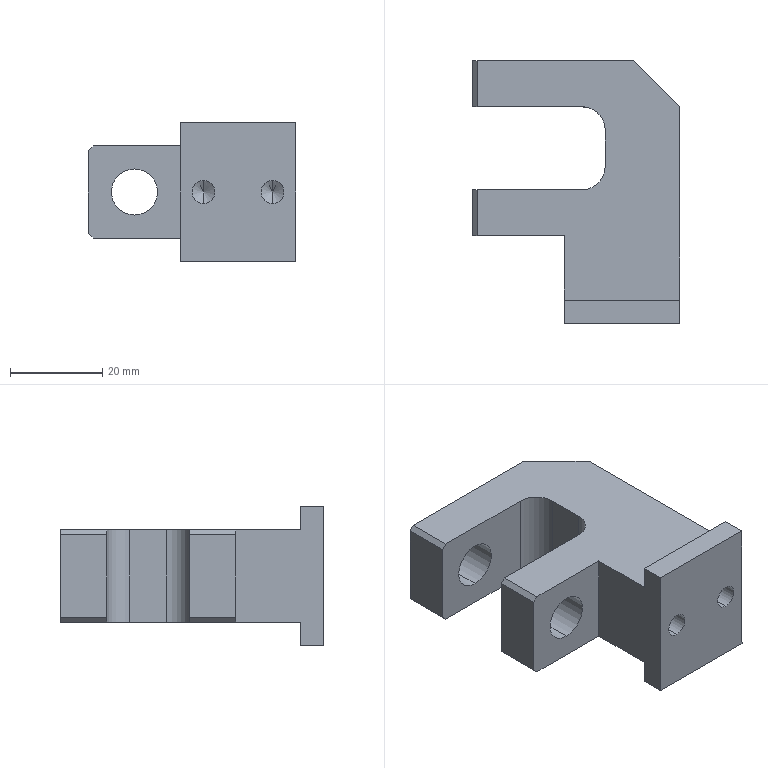Part | SolidWorks | features ICE 4, HoleWzd 3, Chamfer 2, Extrusion 1, Fillet 1 | 1 solid | 35 faces | box 45 x 57 x 30 mm | volume 31506 mm3 | plane 21 | cylinder 10 | cone 4 | commonest cylinder face diameters 10 x6 5 x4
STEP:
#1=CARTESIAN_POINT('',(-2.855,17.,2.5));
#2=VERTEX_POINT('',#1);
#3=CARTESIAN_POINT('',(-2.855,17.,-2.5));
#4=VERTEX_POINT('',#3);
#5=CARTESIAN_POINT('',(-2.855,17.,0.));
#6=DIRECTION('',(0.,-1.,0.));
#7=DIRECTION('',(0.,0.,-1.));
#8=AXIS2_PLACEMENT_3D('',#5,#6,#7);
#9=CIRCLE('',#8,2.5);
#10=EDGE_CURVE('',#2,#4,#9,.T.);
#11=ORIENTED_EDGE('',*,*,#10,.F.);
#12=CARTESIAN_POINT('',(-2.855,0.,2.5));
#13=VERTEX_POINT('',#12);
#14=CARTESIAN_POINT('',(-2.855,0.,2.5));
#15=DIRECTION('',(0.,-1.,0.));
#16=VECTOR('',#15,1000.);
#17=LINE('',#14,#16);
#18=EDGE_CURVE('',#2,#13,#17,.T.);
#19=ORIENTED_EDGE('',*,*,#18,.T.);
#20=CARTESIAN_POINT('',(-2.855,0.,-2.5));
#21=VERTEX_POINT('',#20);
#22=CARTESIAN_POINT('',(-2.855,0.,0.));
#23=DIRECTION('',(0.,-1.,0.));
#24=DIRECTION('',(0.,0.,-1.));
#25=AXIS2_PLACEMENT_3D('',#22,#23,#24);
#26=CIRCLE('',#25,2.5);
#27=EDGE_CURVE('',#13,#21,#26,.T.);
#28=ORIENTED_EDGE('',*,*,#27,.T.);
#29=CARTESIAN_POINT('',(-2.855,0.,-2.5));
#30=DIRECTION('',(0.,-1.,0.));
#31=VECTOR('',#30,1000.);
#32=LINE('',#29,#31);
#33=EDGE_CURVE('',#4,#21,#32,.T.);
#34=ORIENTED_EDGE('',*,*,#33,.F.);
#35=EDGE_LOOP('',(#11,#19,#28,#34));
#36=FACE_OUTER_BOUND('',#35,.T.);
#37=CARTESIAN_POINT('',(-2.855,0.,0.));
#38=DIRECTION('',(0.,-1.,0.));
#39=DIRECTION('',(0.,0.,-1.));
#40=AXIS2_PLACEMENT_3D('',#37,#38,#39);
#41=CYLINDRICAL_SURFACE('',#40,2.5);
#42=ADVANCED_FACE('',(#36),#41,.F.);
#43=CARTESIAN_POINT('',(-2.855,18.502,0.));
#44=VERTEX_POINT('',#43);
#45=CARTESIAN_POINT('',(-2.855,17.,-2.5));
#46=DIRECTION('',(0.,-0.515,-0.8572));
#47=VECTOR('',#46,1000.);
#48=LINE('',#45,#47);
#49=EDGE_CURVE('',#44,#4,#48,.T.);
#50=ORIENTED_EDGE('',*,*,#49,.F.);
#51=CARTESIAN_POINT('',(-2.855,17.,2.5));
#52=DIRECTION('',(0.,-0.515,0.8572));
#53=VECTOR('',#52,1000.);
#54=LINE('',#51,#53);
#55=EDGE_CURVE('',#44,#2,#54,.T.);
#56=ORIENTED_EDGE('',*,*,#55,.T.);
#57=ORIENTED_EDGE('',*,*,#10,.T.);
#58=EDGE_LOOP('',(#50,#56,#57));
#59=FACE_OUTER_BOUND('',#58,.T.);
#60=CARTESIAN_POINT('',(-2.855,17.,0.));
#61=DIRECTION('',(0.,-1.,0.));
#62=DIRECTION('',(0.,0.,-1.));
#63=AXIS2_PLACEMENT_3D('',#60,#61,#62);
#64=CONICAL_SURFACE('',#63,2.5,1.03);
#65=ADVANCED_FACE('',(#59),#64,.F.);
#66=CARTESIAN_POINT('',(12.145,17.,2.5));
#67=VERTEX_POINT('',#66);
#68=CARTESIAN_POINT('',(12.145,17.,-2.5));
#69=VERTEX_POINT('',#68);
#70=CARTESIAN_POINT('',(12.145,17.,0.));
#71=DIRECTION('',(0.,-1.,0.));
#72=DIRECTION('',(0.,0.,-1.));
#73=AXIS2_PLACEMENT_3D('',#70,#71,#72);
#74=CIRCLE('',#73,2.5);
#75=EDGE_CURVE('',#67,#69,#74,.T.);
#76=ORIENTED_EDGE('',*,*,#75,.F.);
#77=CARTESIAN_POINT('',(12.145,0.,2.5));
#78=VERTEX_POINT('',#77);
#79=CARTESIAN_POINT('',(12.145,0.,2.5));
#80=DIRECTION('',(0.,-1.,0.));
#81=VECTOR('',#80,1000.);
#82=LINE('',#79,#81);
#83=EDGE_CURVE('',#67,#78,#82,.T.);
#84=ORIENTED_EDGE('',*,*,#83,.T.);
#85=CARTESIAN_POINT('',(12.145,0.,-2.5));
#86=VERTEX_POINT('',#85);
#87=CARTESIAN_POINT('',(12.145,0.,0.));
#88=DIRECTION('',(0.,-1.,0.));
#89=DIRECTION('',(0.,0.,-1.));
#90=AXIS2_PLACEMENT_3D('',#87,#88,#89);
#91=CIRCLE('',#90,2.5);
#92=EDGE_CURVE('',#78,#86,#91,.T.);
#93=ORIENTED_EDGE('',*,*,#92,.T.);
#94=CARTESIAN_POINT('',(12.145,0.,-2.5));
#95=DIRECTION('',(0.,-1.,0.));
#96=VECTOR('',#95,1000.);
#97=LINE('',#94,#96);
#98=EDGE_CURVE('',#69,#86,#97,.T.);
#99=ORIENTED_EDGE('',*,*,#98,.F.);
#100=EDGE_LOOP('',(#76,#84,#93,#99));
#101=FACE_OUTER_BOUND('',#100,.T.);
#102=CARTESIAN_POINT('',(12.145,0.,0.));
#103=DIRECTION('',(0.,-1.,0.));
#104=DIRECTION('',(0.,0.,-1.));
#105=AXIS2_PLACEMENT_3D('',#102,#103,#104);
#106=CYLINDRICAL_SURFACE('',#105,2.5);
#107=ADVANCED_FACE('',(#101),#106,.F.);
#108=CARTESIAN_POINT('',(12.145,18.502,0.));
#109=VERTEX_POINT('',#108);
#110=CARTESIAN_POINT('',(12.145,17.,-2.5));
#111=DIRECTION('',(0.,-0.515,-0.8572));
#112=VECTOR('',#111,1000.);
#113=LINE('',#110,#112);
#114=EDGE_CURVE('',#109,#69,#113,.T.);
#115=ORIENTED_EDGE('',*,*,#114,.F.);
#116=CARTESIAN_POINT('',(12.145,17.,2.5));
#117=DIRECTION('',(0.,-0.515,0.8572));
#118=VECTOR('',#117,1000.);
#119=LINE('',#116,#118);
#120=EDGE_CURVE('',#109,#67,#119,.T.);
#121=ORIENTED_EDGE('',*,*,#120,.T.);
#122=ORIENTED_EDGE('',*,*,#75,.T.);
#123=EDGE_LOOP('',(#115,#121,#122));
#124=FACE_OUTER_BOUND('',#123,.T.);
#125=CARTESIAN_POINT('',(12.145,17.,0.));
#126=DIRECTION('',(0.,-1.,0.));
#127=DIRECTION('',(0.,0.,-1.));
#128=AXIS2_PLACEMENT_3D('',#125,#126,#127);
#129=CONICAL_SURFACE('',#128,2.5,1.03);
#130=ADVANCED_FACE('',(#124),#129,.F.);
#131=CARTESIAN_POINT('',(-17.855,29.,5.));
#132=VERTEX_POINT('',#131);
#133=CARTESIAN_POINT('',(-17.855,29.,-5.));
#134=VERTEX_POINT('',#133);
#135=CARTESIAN_POINT('',(-17.855,29.,0.));
#136=DIRECTION('',(0.,-1.,0.));
#137=DIRECTION('',(0.,0.,-1.));
#138=AXIS2_PLACEMENT_3D('',#135,#136,#137);
#139=CIRCLE('',#138,5.);
#140=EDGE_CURVE('',#132,#134,#139,.T.);
#141=ORIENTED_EDGE('',*,*,#140,.F.);
#142=CARTESIAN_POINT('',(-17.855,19.,5.));
#143=VERTEX_POINT('',#142);
#144=CARTESIAN_POINT('',(-17.855,19.,5.));
#145=DIRECTION('',(0.,-1.,0.));
#146=VECTOR('',#145,1000.);
#147=LINE('',#144,#146);
#148=EDGE_CURVE('',#132,#143,#147,.T.);
#149=ORIENTED_EDGE('',*,*,#148,.T.);
#150=CARTESIAN_POINT('',(-17.855,19.,-5.));
#151=VERTEX_POINT('',#150);
#152=CARTESIAN_POINT('',(-17.855,19.,0.));
#153=DIRECTION('',(0.,-1.,0.));
#154=DIRECTION('',(0.,0.,-1.));
#155=AXIS2_PLACEMENT_3D('',#152,#153,#154);
#156=CIRCLE('',#155,5.);
#157=EDGE_CURVE('',#143,#151,#156,.T.);
#158=ORIENTED_EDGE('',*,*,#157,.T.);
#159=CARTESIAN_POINT('',(-17.855,19.,-5.));
#160=DIRECTION('',(0.,-1.,0.));
#161=VECTOR('',#160,1000.);
#162=LINE('',#159,#161);
#163=EDGE_CURVE('',#134,#151,#162,.T.);
#164=ORIENTED_EDGE('',*,*,#163,.F.);
#165=EDGE_LOOP('',(#141,#149,#158,#164));
#166=FACE_OUTER_BOUND('',#165,.T.);
#167=CARTESIAN_POINT('',(-17.855,19.,0.));
#168=DIRECTION('',(0.,-1.,0.));
#169=DIRECTION('',(0.,0.,-1.));
#170=AXIS2_PLACEMENT_3D('',#167,#168,#169);
#171=CYLINDRICAL_SURFACE('',#170,5.);
#172=ADVANCED_FACE('',(#166),#171,.F.);
#173=CARTESIAN_POINT('',(-17.855,57.,5.));
#174=VERTEX_POINT('',#173);
#175=CARTESIAN_POINT('',(-17.855,57.,-5.));
#176=VERTEX_POINT('',#175);
#177=CARTESIAN_POINT('',(-17.855,57.,0.));
#178=DIRECTION('',(0.,-1.,0.));
#179=DIRECTION('',(0.,0.,-1.));
#180=AXIS2_PLACEMENT_3D('',#177,#178,#179);
#181=CIRCLE('',#180,5.);
#182=EDGE_CURVE('',#174,#176,#181,.T.);
#183=ORIENTED_EDGE('',*,*,#182,.F.);
#184=CARTESIAN_POINT('',(-17.855,47.,5.));
#185=VERTEX_POINT('',#184);
#186=CARTESIAN_POINT('',(-17.855,47.,5.));
#187=DIRECTION('',(0.,-1.,0.));
#188=VECTOR('',#187,1000.);
#189=LINE('',#186,#188);
#190=EDGE_CURVE('',#174,#185,#189,.T.);
#191=ORIENTED_EDGE('',*,*,#190,.T.);
#192=CARTESIAN_POINT('',(-17.855,47.,-5.));
#193=VERTEX_POINT('',#192);
#194=CARTESIAN_POINT('',(-17.855,47.,0.));
#195=DIRECTION('',(0.,-1.,0.));
#196=DIRECTION('',(0.,0.,-1.));
#197=AXIS2_PLACEMENT_3D('',#194,#195,#196);
#198=CIRCLE('',#197,5.);
#199=EDGE_CURVE('',#185,#193,#198,.T.);
#200=ORIENTED_EDGE('',*,*,#199,.T.);
#201=CARTESIAN_POINT('',(-17.855,47.,-5.));
#202=DIRECTION('',(0.,-1.,0.));
#203=VECTOR('',#202,1000.);
#204=LINE('',#201,#203);
#205=EDGE_CURVE('',#176,#193,#204,.T.);
#206=ORIENTED_EDGE('',*,*,#205,.F.);
#207=EDGE_LOOP('',(#183,#191,#200,#206));
#208=FACE_OUTER_BOUND('',#207,.T.);
#209=CARTESIAN_POINT('',(-17.855,47.,0.));
#210=DIRECTION('',(0.,-1.,0.));
#211=DIRECTION('',(0.,0.,-1.));
#212=AXIS2_PLACEMENT_3D('',#209,#210,#211);
#213=CYLINDRICAL_SURFACE('',#212,5.);
#214=ADVANCED_FACE('',(#208),#213,.F.);
#215=CARTESIAN_POINT('',(-27.855,57.,9.));
#216=VERTEX_POINT('',#215);
#217=CARTESIAN_POINT('',(-27.855,57.,-9.));
#218=VERTEX_POINT('',#217);
#219=CARTESIAN_POINT('',(-27.855,57.,-10.));
#220=DIRECTION('',(0.,0.,-1.));
#221=VECTOR('',#220,1000.);
#222=LINE('',#219,#221);
#223=EDGE_CURVE('',#216,#218,#222,.T.);
#224=ORIENTED_EDGE('',*,*,#223,.T.);
#225=CARTESIAN_POINT('',(-27.855,47.,-9.));
#226=VERTEX_POINT('',#225);
#227=CARTESIAN_POINT('',(-27.855,0.,-9.));
#228=DIRECTION('',(0.,-1.,0.));
#229=VECTOR('',#228,1000.);
#230=LINE('',#227,#229);
#231=EDGE_CURVE('',#218,#226,#230,.T.);
#232=ORIENTED_EDGE('',*,*,#231,.T.);
#233=CARTESIAN_POINT('',(-27.855,47.,9.));
#234=VERTEX_POINT('',#233);
#235=CARTESIAN_POINT('',(-27.855,47.,0.));
#236=DIRECTION('',(0.,0.,1.));
#237=VECTOR('',#236,1000.);
#238=LINE('',#235,#237);
#239=EDGE_CURVE('',#226,#234,#238,.T.);
#240=ORIENTED_EDGE('',*,*,#239,.T.);
#241=CARTESIAN_POINT('',(-27.855,0.,9.));
#242=DIRECTION('',(0.,1.,0.));
#243=VECTOR('',#242,1000.);
#244=LINE('',#241,#243);
#245=EDGE_CURVE('',#234,#216,#244,.T.);
#246=ORIENTED_EDGE('',*,*,#245,.T.);
#247=EDGE_LOOP('',(#224,#232,#240,#246));
#248=FACE_OUTER_BOUND('',#247,.T.);
#249=CARTESIAN_POINT('',(-27.855,0.,0.));
#250=DIRECTION('',(1.,0.,0.));
#251=DIRECTION('',(0.,0.,-1.));
#252=AXIS2_PLACEMENT_3D('',#249,#250,#251);
#253=PLANE('',#252);
#254=ADVANCED_FACE('',(#248),#253,.F.);
#255=CARTESIAN_POINT('',(-7.855,19.,-10.));
#256=VERTEX_POINT('',#255);
#257=CARTESIAN_POINT('',(-7.855,19.,10.));
#258=VERTEX_POINT('',#257);
#259=CARTESIAN_POINT('',(-7.855,19.,10.));
#260=DIRECTION('',(0.,0.,1.));
#261=VECTOR('',#260,1000.);
#262=LINE('',#259,#261);
#263=EDGE_CURVE('',#256,#258,#262,.T.);
#264=ORIENTED_EDGE('',*,*,#263,.F.);
#265=CARTESIAN_POINT('',(-7.855,5.,-10.));
#266=VERTEX_POINT('',#265);
#267=CARTESIAN_POINT('',(-7.855,57.,-10.));
#268=DIRECTION('',(0.,-1.,0.));
#269=VECTOR('',#268,1000.);
#270=LINE('',#267,#269);
#271=EDGE_CURVE('',#256,#266,#270,.T.);
#272=ORIENTED_EDGE('',*,*,#271,.T.);
#273=CARTESIAN_POINT('',(-7.855,5.,-15.));
#274=VERTEX_POINT('',#273);
#275=CARTESIAN_POINT('',(-7.855,5.,-10.));
#276=DIRECTION('',(0.,0.,-1.));
#277=VECTOR('',#276,1000.);
#278=LINE('',#275,#277);
#279=EDGE_CURVE('',#266,#274,#278,.T.);
#280=ORIENTED_EDGE('',*,*,#279,.T.);
#281=CARTESIAN_POINT('',(-7.855,0.,-15.));
#282=VERTEX_POINT('',#281);
#283=CARTESIAN_POINT('',(-7.855,0.,-15.));
#284=DIRECTION('',(0.,1.,0.));
#285=VECTOR('',#284,1000.);
#286=LINE('',#283,#285);
#287=EDGE_CURVE('',#282,#274,#286,.T.);
#288=ORIENTED_EDGE('',*,*,#287,.F.);
#289=CARTESIAN_POINT('',(-7.855,0.,15.));
#290=VERTEX_POINT('',#289);
#291=CARTESIAN_POINT('',(-7.855,0.,15.));
#292=DIRECTION('',(0.,0.,-1.));
#293=VECTOR('',#292,1000.);
#294=LINE('',#291,#293);
#295=EDGE_CURVE('',#290,#282,#294,.T.);
#296=ORIENTED_EDGE('',*,*,#295,.F.);
#297=CARTESIAN_POINT('',(-7.855,5.,15.));
#298=VERTEX_POINT('',#297);
#299=CARTESIAN_POINT('',(-7.855,57.,15.));
#300=DIRECTION('',(0.,-1.,0.));
#301=VECTOR('',#300,1000.);
#302=LINE('',#299,#301);
#303=EDGE_CURVE('',#298,#290,#302,.T.);
#304=ORIENTED_EDGE('',*,*,#303,.F.);
#305=CARTESIAN_POINT('',(-7.855,5.,10.));
#306=VERTEX_POINT('',#305);
#307=CARTESIAN_POINT('',(-7.855,5.,15.));
#308=DIRECTION('',(0.,0.,-1.));
#309=VECTOR('',#308,1000.);
#310=LINE('',#307,#309);
#311=EDGE_CURVE('',#298,#306,#310,.T.);
#312=ORIENTED_EDGE('',*,*,#311,.T.);
#313=CARTESIAN_POINT('',(-7.855,5.,10.));
#314=DIRECTION('',(0.,1.,0.));
#315=VECTOR('',#314,1000.);
#316=LINE('',#313,#315);
#317=EDGE_CURVE('',#306,#258,#316,.T.);
#318=ORIENTED_EDGE('',*,*,#317,.T.);
#319=EDGE_LOOP('',(#264,#272,#280,#288,#296,#304,#312,#318));
#320=FACE_OUTER_BOUND('',#319,.T.);
#321=CARTESIAN_POINT('',(-7.855,0.,0.));
#322=DIRECTION('',(1.,0.,0.));
#323=DIRECTION('',(0.,0.,-1.));
#324=AXIS2_PLACEMENT_3D('',#321,#322,#323);
#325=PLANE('',#324);
#326=ADVANCED_FACE('',(#320),#325,.F.);
#327=CARTESIAN_POINT('',(17.145,5.,-15.));
#328=VERTEX_POINT('',#327);
#329=CARTESIAN_POINT('',(-7.855,5.,-15.));
#330=DIRECTION('',(1.,0.,0.));
#331=VECTOR('',#330,1000.);
#332=LINE('',#329,#331);
#333=EDGE_CURVE('',#274,#328,#332,.T.);
#334=ORIENTED_EDGE('',*,*,#333,.T.);
#335=CARTESIAN_POINT('',(17.145,0.,-15.));
#336=VERTEX_POINT('',#335);
#337=CARTESIAN_POINT('',(17.145,0.,-15.));
#338=DIRECTION('',(0.,1.,0.));
#339=VECTOR('',#338,1000.);
#340=LINE('',#337,#339);
#341=EDGE_CURVE('',#336,#328,#340,.T.);
#342=ORIENTED_EDGE('',*,*,#341,.F.);
#343=CARTESIAN_POINT('',(-7.855,0.,-15.));
#344=DIRECTION('',(1.,0.,0.));
#345=VECTOR('',#344,1000.);
#346=LINE('',#343,#345);
#347=EDGE_CURVE('',#282,#336,#346,.T.);
#348=ORIENTED_EDGE('',*,*,#347,.F.);
#349=ORIENTED_EDGE('',*,*,#287,.T.);
#350=EDGE_LOOP('',(#334,#342,#348,#349));
#351=FACE_OUTER_BOUND('',#350,.T.);
#352=CARTESIAN_POINT('',(-7.855,0.,-15.));
#353=DIRECTION('',(0.,0.,-1.));
#354=DIRECTION('',(-1.,0.,0.));
#355=AXIS2_PLACEMENT_3D('',#352,#353,#354);
#356=PLANE('',#355);
#357=ADVANCED_FACE('',(#351),#356,.T.);
#358=CARTESIAN_POINT('',(-2.855,0.,0.));
#359=DIRECTION('',(0.,-1.,0.));
#360=DIRECTION('',(0.,0.,-1.));
#361=AXIS2_PLACEMENT_3D('',#358,#359,#360);
#362=CIRCLE('',#361,2.5);
#363=EDGE_CURVE('',#21,#13,#362,.T.);
#364=ORIENTED_EDGE('',*,*,#363,.F.);
#365=ORIENTED_EDGE('',*,*,#27,.F.);
#366=EDGE_LOOP('',(#364,#365));
#367=FACE_BOUND('',#366,.T.);
#368=CARTESIAN_POINT('',(12.145,0.,0.));
#369=DIRECTION('',(0.,-1.,0.));
#370=DIRECTION('',(0.,0.,-1.));
#371=AXIS2_PLACEMENT_3D('',#368,#369,#370);
#372=CIRCLE('',#371,2.5);
#373=EDGE_CURVE('',#86,#78,#372,.T.);
#374=ORIENTED_EDGE('',*,*,#373,.F.);
#375=ORIENTED_EDGE('',*,*,#92,.F.);
#376=EDGE_LOOP('',(#374,#375));
#377=FACE_BOUND('',#376,.T.);
#378=CARTESIAN_POINT('',(17.145,0.,15.));
#379=VERTEX_POINT('',#378);
#380=CARTESIAN_POINT('',(17.145,0.,15.));
#381=DIRECTION('',(0.,0.,-1.));
#382=VECTOR('',#381,1000.);
#383=LINE('',#380,#382);
#384=EDGE_CURVE('',#379,#336,#383,.T.);
#385=ORIENTED_EDGE('',*,*,#384,.F.);
#386=CARTESIAN_POINT('',(-7.855,0.,15.));
#387=DIRECTION('',(1.,0.,0.));
#388=VECTOR('',#387,1000.);
#389=LINE('',#386,#388);
#390=EDGE_CURVE('',#290,#379,#389,.T.);
#391=ORIENTED_EDGE('',*,*,#390,.F.);
#392=ORIENTED_EDGE('',*,*,#295,.T.);
#393=ORIENTED_EDGE('',*,*,#347,.T.);
#394=EDGE_LOOP('',(#385,#391,#392,#393));
#395=FACE_OUTER_BOUND('',#394,.T.);
#396=CARTESIAN_POINT('',(-7.855,0.,15.));
#397=DIRECTION('',(0.,-1.,0.));
#398=DIRECTION('',(0.,0.,-1.));
#399=AXIS2_PLACEMENT_3D('',#396,#397,#398);
#400=PLANE('',#399);
#401=ADVANCED_FACE('',(#367,#377,#395),#400,.T.);
#402=CARTESIAN_POINT('',(17.145,5.,15.));
#403=VERTEX_POINT('',#402);
#404=CARTESIAN_POINT('',(-7.855,5.,15.));
#405=DIRECTION('',(1.,0.,0.));
#406=VECTOR('',#405,1000.);
#407=LINE('',#404,#406);
#408=EDGE_CURVE('',#298,#403,#407,.T.);
#409=ORIENTED_EDGE('',*,*,#408,.F.);
#410=ORIENTED_EDGE('',*,*,#303,.T.);
#411=ORIENTED_EDGE('',*,*,#390,.T.);
#412=CARTESIAN_POINT('',(17.145,57.,15.));
#413=DIRECTION('',(0.,-1.,0.));
#414=VECTOR('',#413,1000.);
#415=LINE('',#412,#414);
#416=EDGE_CURVE('',#403,#379,#415,.T.);
#417=ORIENTED_EDGE('',*,*,#416,.F.);
#418=EDGE_LOOP('',(#409,#410,#411,#417));
#419=FACE_OUTER_BOUND('',#418,.T.);
#420=CARTESIAN_POINT('',(-7.855,57.,15.));
#421=DIRECTION('',(0.,0.,1.));
#422=DIRECTION('',(1.,0.,0.));
#423=AXIS2_PLACEMENT_3D('',#420,#421,#422);
#424=PLANE('',#423);
#425=ADVANCED_FACE('',(#419),#424,.T.);
#426=CARTESIAN_POINT('',(-17.855,57.,0.));
#427=DIRECTION('',(0.,-1.,0.));
#428=DIRECTION('',(0.,0.,-1.));
#429=AXIS2_PLACEMENT_3D('',#426,#427,#428);
#430=CIRCLE('',#429,5.);
#431=EDGE_CURVE('',#176,#174,#430,.T.);
#432=ORIENTED_EDGE('',*,*,#431,.T.);
#433=ORIENTED_EDGE('',*,*,#182,.T.);
#434=EDGE_LOOP('',(#432,#433));
#435=FACE_BOUND('',#434,.T.);
#436=CARTESIAN_POINT('',(-26.855,57.,10.));
#437=VERTEX_POINT('',#436);
#438=CARTESIAN_POINT('',(7.145,57.,10.));
#439=VERTEX_POINT('',#438);
#440=CARTESIAN_POINT('',(-7.855,57.,10.));
#441=DIRECTION('',(1.,0.,0.));
#442=VECTOR('',#441,1000.);
#443=LINE('',#440,#442);
#444=EDGE_CURVE('',#437,#439,#443,.T.);
#445=ORIENTED_EDGE('',*,*,#444,.T.);
#446=CARTESIAN_POINT('',(7.145,57.,-10.));
#447=VERTEX_POINT('',#446);
#448=CARTESIAN_POINT('',(7.145,57.,-15.));
#449=DIRECTION('',(0.,0.,-1.));
#450=VECTOR('',#449,1000.);
#451=LINE('',#448,#450);
#452=EDGE_CURVE('',#439,#447,#451,.T.);
#453=ORIENTED_EDGE('',*,*,#452,.T.);
#454=CARTESIAN_POINT('',(-26.855,57.,-10.));
#455=VERTEX_POINT('',#454);
#456=CARTESIAN_POINT('',(-7.855,57.,-10.));
#457=DIRECTION('',(1.,0.,0.));
#458=VECTOR('',#457,1000.);
#459=LINE('',#456,#458);
#460=EDGE_CURVE('',#455,#447,#459,.T.);
#461=ORIENTED_EDGE('',*,*,#460,.F.);
#462=CARTESIAN_POINT('',(-14.855,57.,-22.));
#463=DIRECTION('',(-0.7071,0.,0.7071));
#464=VECTOR('',#463,1000.);
#465=LINE('',#462,#464);
#466=EDGE_CURVE('',#455,#218,#465,.T.);
#467=ORIENTED_EDGE('',*,*,#466,.T.);
#468=ORIENTED_EDGE('',*,*,#223,.F.);
#469=CARTESIAN_POINT('',(-29.855,57.,7.));
#470=DIRECTION('',(0.7071,0.,0.7071));
#471=VECTOR('',#470,1000.);
#472=LINE('',#469,#471);
#473=EDGE_CURVE('',#216,#437,#472,.T.);
#474=ORIENTED_EDGE('',*,*,#473,.T.);
#475=EDGE_LOOP('',(#445,#453,#461,#467,#468,#474));
#476=FACE_OUTER_BOUND('',#475,.T.);
#477=CARTESIAN_POINT('',(-7.855,57.,-15.));
#478=DIRECTION('',(0.,1.,0.));
#479=DIRECTION('',(0.,0.,1.));
#480=AXIS2_PLACEMENT_3D('',#477,#478,#479);
#481=PLANE('',#480);
#482=ADVANCED_FACE('',(#435,#476),#481,.T.);
#483=CARTESIAN_POINT('',(17.145,47.,-10.));
#484=VERTEX_POINT('',#483);
#485=CARTESIAN_POINT('',(17.145,5.,-10.));
#486=VERTEX_POINT('',#485);
#487=CARTESIAN_POINT('',(17.145,57.,-10.));
#488=DIRECTION('',(0.,-1.,0.));
#489=VECTOR('',#488,1000.);
#490=LINE('',#487,#489);
#491=EDGE_CURVE('',#484,#486,#490,.T.);
#492=ORIENTED_EDGE('',*,*,#491,.F.);
#493=CARTESIAN_POINT('',(17.145,47.,10.));
#494=VERTEX_POINT('',#493);
#495=CARTESIAN_POINT('',(17.145,47.,0.));
#496=DIRECTION('',(0.,0.,1.));
#497=VECTOR('',#496,1000.);
#498=LINE('',#495,#497);
#499=EDGE_CURVE('',#484,#494,#498,.T.);
#500=ORIENTED_EDGE('',*,*,#499,.T.);
#501=CARTESIAN_POINT('',(17.145,5.,10.));
#502=VERTEX_POINT('',#501);
#503=CARTESIAN_POINT('',(17.145,5.,10.));
#504=DIRECTION('',(0.,1.,0.));
#505=VECTOR('',#504,1000.);
#506=LINE('',#503,#505);
#507=EDGE_CURVE('',#502,#494,#506,.T.);
#508=ORIENTED_EDGE('',*,*,#507,.F.);
#509=CARTESIAN_POINT('',(17.145,5.,15.));
#510=DIRECTION('',(0.,0.,-1.));
#511=VECTOR('',#510,1000.);
#512=LINE('',#509,#511);
#513=EDGE_CURVE('',#403,#502,#512,.T.);
#514=ORIENTED_EDGE('',*,*,#513,.F.);
#515=ORIENTED_EDGE('',*,*,#416,.T.);
#516=ORIENTED_EDGE('',*,*,#384,.T.);
#517=ORIENTED_EDGE('',*,*,#341,.T.);
#518=CARTESIAN_POINT('',(17.145,5.,-10.));
#519=DIRECTION('',(0.,0.,-1.));
#520=VECTOR('',#519,1000.);
#521=LINE('',#518,#520);
#522=EDGE_CURVE('',#486,#328,#521,.T.);
#523=ORIENTED_EDGE('',*,*,#522,.F.);
#524=EDGE_LOOP('',(#492,#500,#508,#514,#515,#516,#517,#523));
#525=FACE_OUTER_BOUND('',#524,.T.);
#526=CARTESIAN_POINT('',(17.145,0.,0.));
#527=DIRECTION('',(1.,0.,0.));
#528=DIRECTION('',(0.,0.,-1.));
#529=AXIS2_PLACEMENT_3D('',#526,#527,#528);
#530=PLANE('',#529);
#531=ADVANCED_FACE('',(#525),#530,.T.);
#532=ORIENTED_EDGE('',*,*,#507,.T.);
#533=CARTESIAN_POINT('',(17.145,47.,10.));
#534=DIRECTION('',(-0.7071,0.7071,0.));
#535=VECTOR('',#534,1000.);
#536=LINE('',#533,#535);
#537=EDGE_CURVE('',#494,#439,#536,.T.);
#538=ORIENTED_EDGE('',*,*,#537,.T.);
#539=ORIENTED_EDGE('',*,*,#444,.F.);
#540=CARTESIAN_POINT('',(-26.855,47.,10.));
#541=VERTEX_POINT('',#540);
#542=CARTESIAN_POINT('',(-26.855,5.,10.));
#543=DIRECTION('',(0.,-1.,0.));
#544=VECTOR('',#543,1000.);
#545=LINE('',#542,#544);
#546=EDGE_CURVE('',#437,#541,#545,.T.);
#547=ORIENTED_EDGE('',*,*,#546,.T.);
#548=CARTESIAN_POINT('',(-4.018,47.,10.));
#549=VERTEX_POINT('',#548);
#550=CARTESIAN_POINT('',(0.9816,47.,10.));
#551=DIRECTION('',(-1.,0.,0.));
#552=VECTOR('',#551,1000.);
#553=LINE('',#550,#552);
#554=EDGE_CURVE('',#549,#541,#553,.T.);
#555=ORIENTED_EDGE('',*,*,#554,.F.);
#556=CARTESIAN_POINT('',(0.9816,42.,10.));
#557=VERTEX_POINT('',#556);
#558=CARTESIAN_POINT('',(-4.018,42.,10.));
#559=DIRECTION('',(0.,0.,-1.));
#560=DIRECTION('',(-1.,0.,0.));
#561=AXIS2_PLACEMENT_3D('',#558,#559,#560);
#562=CIRCLE('',#561,5.);
#563=EDGE_CURVE('',#549,#557,#562,.T.);
#564=ORIENTED_EDGE('',*,*,#563,.T.);
#565=CARTESIAN_POINT('',(0.9816,34.,10.));
#566=VERTEX_POINT('',#565);
#567=CARTESIAN_POINT('',(0.9816,29.,10.));
#568=DIRECTION('',(0.,1.,0.));
#569=VECTOR('',#568,1000.);
#570=LINE('',#567,#569);
#571=EDGE_CURVE('',#566,#557,#570,.T.);
#572=ORIENTED_EDGE('',*,*,#571,.F.);
#573=CARTESIAN_POINT('',(-4.018,29.,10.));
#574=VERTEX_POINT('',#573);
#575=CARTESIAN_POINT('',(-4.018,34.,10.));
#576=DIRECTION('',(0.,0.,-1.));
#577=DIRECTION('',(-1.,0.,0.));
#578=AXIS2_PLACEMENT_3D('',#575,#576,#577);
#579=CIRCLE('',#578,5.);
#580=EDGE_CURVE('',#566,#574,#579,.T.);
#581=ORIENTED_EDGE('',*,*,#580,.T.);
#582=CARTESIAN_POINT('',(-26.855,29.,10.));
#583=VERTEX_POINT('',#582);
#584=CARTESIAN_POINT('',(-27.855,29.,10.));
#585=DIRECTION('',(1.,0.,0.));
#586=VECTOR('',#585,1000.);
#587=LINE('',#584,#586);
#588=EDGE_CURVE('',#583,#574,#587,.T.);
#589=ORIENTED_EDGE('',*,*,#588,.F.);
#590=CARTESIAN_POINT('',(-26.855,19.,10.));
#591=VERTEX_POINT('',#590);
#592=CARTESIAN_POINT('',(-26.855,5.,10.));
#593=DIRECTION('',(0.,-1.,0.));
#594=VECTOR('',#593,1000.);
#595=LINE('',#592,#594);
#596=EDGE_CURVE('',#583,#591,#595,.T.);
#597=ORIENTED_EDGE('',*,*,#596,.T.);
#598=CARTESIAN_POINT('',(-27.855,19.,10.));
#599=DIRECTION('',(1.,0.,0.));
#600=VECTOR('',#599,1000.);
#601=LINE('',#598,#600);
#602=EDGE_CURVE('',#591,#258,#601,.T.);
#603=ORIENTED_EDGE('',*,*,#602,.T.);
#604=ORIENTED_EDGE('',*,*,#317,.F.);
#605=CARTESIAN_POINT('',(-7.855,5.,10.));
#606=DIRECTION('',(1.,0.,0.));
#607=VECTOR('',#606,1000.);
#608=LINE('',#605,#607);
#609=EDGE_CURVE('',#306,#502,#608,.T.);
#610=ORIENTED_EDGE('',*,*,#609,.T.);
#611=EDGE_LOOP('',(#532,#538,#539,#547,#555,#564,#572,#581,#589,#597,#603,#604,#610));
#612=FACE_OUTER_BOUND('',#611,.T.);
#613=CARTESIAN_POINT('',(-7.855,5.,10.));
#614=DIRECTION('',(0.,0.,-1.));
#615=DIRECTION('',(-1.,0.,0.));
#616=AXIS2_PLACEMENT_3D('',#613,#614,#615);
#617=PLANE('',#616);
#618=ADVANCED_FACE('',(#612),#617,.F.);
#619=ORIENTED_EDGE('',*,*,#513,.T.);
#620=ORIENTED_EDGE('',*,*,#609,.F.);
#621=ORIENTED_EDGE('',*,*,#311,.F.);
#622=ORIENTED_EDGE('',*,*,#408,.T.);
#623=EDGE_LOOP('',(#619,#620,#621,#622));
#624=FACE_OUTER_BOUND('',#623,.T.);
#625=CARTESIAN_POINT('',(-7.855,5.,15.));
#626=DIRECTION('',(0.,-1.,0.));
#627=DIRECTION('',(0.,0.,-1.));
#628=AXIS2_PLACEMENT_3D('',#625,#626,#627);
#629=PLANE('',#628);
#630=ADVANCED_FACE('',(#624),#629,.F.);
#631=ORIENTED_EDGE('',*,*,#460,.T.);
#632=CARTESIAN_POINT('',(17.145,47.,-10.));
#633=DIRECTION('',(0.7071,-0.7071,0.));
#634=VECTOR('',#633,1000.);
#635=LINE('',#632,#634);
#636=EDGE_CURVE('',#447,#484,#635,.T.);
#637=ORIENTED_EDGE('',*,*,#636,.T.);
#638=ORIENTED_EDGE('',*,*,#491,.T.);
#639=CARTESIAN_POINT('',(-7.855,5.,-10.));
#640=DIRECTION('',(1.,0.,0.));
#641=VECTOR('',#640,1000.);
#642=LINE('',#639,#641);
#643=EDGE_CURVE('',#266,#486,#642,.T.);
#644=ORIENTED_EDGE('',*,*,#643,.F.);
#645=ORIENTED_EDGE('',*,*,#271,.F.);
#646=CARTESIAN_POINT('',(-26.855,19.,-10.));
#647=VERTEX_POINT('',#646);
#648=CARTESIAN_POINT('',(-27.855,19.,-10.));
#649=DIRECTION('',(1.,0.,0.));
#650=VECTOR('',#649,1000.);
#651=LINE('',#648,#650);
#652=EDGE_CURVE('',#647,#256,#651,.T.);
#653=ORIENTED_EDGE('',*,*,#652,.F.);
#654=CARTESIAN_POINT('',(-26.855,29.,-10.));
#655=VERTEX_POINT('',#654);
#656=CARTESIAN_POINT('',(-26.855,57.,-10.));
#657=DIRECTION('',(0.,1.,0.));
#658=VECTOR('',#657,1000.);
#659=LINE('',#656,#658);
#660=EDGE_CURVE('',#647,#655,#659,.T.);
#661=ORIENTED_EDGE('',*,*,#660,.T.);
#662=CARTESIAN_POINT('',(-4.018,29.,-10.));
#663=VERTEX_POINT('',#662);
#664=CARTESIAN_POINT('',(-7.855,29.,-10.));
#665=DIRECTION('',(1.,0.,0.));
#666=VECTOR('',#665,1000.);
#667=LINE('',#664,#666);
#668=EDGE_CURVE('',#655,#663,#667,.T.);
#669=ORIENTED_EDGE('',*,*,#668,.T.);
#670=CARTESIAN_POINT('',(0.9816,34.,-10.));
#671=VERTEX_POINT('',#670);
#672=CARTESIAN_POINT('',(-4.018,34.,-10.));
#673=DIRECTION('',(0.,0.,1.));
#674=DIRECTION('',(0.,-1.,0.));
#675=AXIS2_PLACEMENT_3D('',#672,#673,#674);
#676=CIRCLE('',#675,5.);
#677=EDGE_CURVE('',#663,#671,#676,.T.);
#678=ORIENTED_EDGE('',*,*,#677,.T.);
#679=CARTESIAN_POINT('',(0.9816,42.,-10.));
#680=VERTEX_POINT('',#679);
#681=CARTESIAN_POINT('',(0.9816,57.,-10.));
#682=DIRECTION('',(0.,1.,0.));
#683=VECTOR('',#682,1000.);
#684=LINE('',#681,#683);
#685=EDGE_CURVE('',#671,#680,#684,.T.);
#686=ORIENTED_EDGE('',*,*,#685,.T.);
#687=CARTESIAN_POINT('',(-4.018,47.,-10.));
#688=VERTEX_POINT('',#687);
#689=CARTESIAN_POINT('',(-4.018,42.,-10.));
#690=DIRECTION('',(0.,0.,1.));
#691=DIRECTION('',(0.,-1.,0.));
#692=AXIS2_PLACEMENT_3D('',#689,#690,#691);
#693=CIRCLE('',#692,5.);
#694=EDGE_CURVE('',#680,#688,#693,.T.);
#695=ORIENTED_EDGE('',*,*,#694,.T.);
#696=CARTESIAN_POINT('',(-26.855,47.,-10.));
#697=VERTEX_POINT('',#696);
#698=CARTESIAN_POINT('',(-7.855,47.,-10.));
#699=DIRECTION('',(-1.,0.,0.));
#700=VECTOR('',#699,1000.);
#701=LINE('',#698,#700);
#702=EDGE_CURVE('',#688,#697,#701,.T.);
#703=ORIENTED_EDGE('',*,*,#702,.T.);
#704=CARTESIAN_POINT('',(-26.855,57.,-10.));
#705=DIRECTION('',(0.,1.,0.));
#706=VECTOR('',#705,1000.);
#707=LINE('',#704,#706);
#708=EDGE_CURVE('',#697,#455,#707,.T.);
#709=ORIENTED_EDGE('',*,*,#708,.T.);
#710=EDGE_LOOP('',(#631,#637,#638,#644,#645,#653,#661,#669,#678,#686,#695,#703,#709));
#711=FACE_OUTER_BOUND('',#710,.T.);
#712=CARTESIAN_POINT('',(-7.855,57.,-10.));
#713=DIRECTION('',(0.,0.,1.));
#714=DIRECTION('',(0.,-1.,0.));
#715=AXIS2_PLACEMENT_3D('',#712,#713,#714);
#716=PLANE('',#715);
#717=ADVANCED_FACE('',(#711),#716,.F.);
#718=ORIENTED_EDGE('',*,*,#522,.T.);
#719=ORIENTED_EDGE('',*,*,#333,.F.);
#720=ORIENTED_EDGE('',*,*,#279,.F.);
#721=ORIENTED_EDGE('',*,*,#643,.T.);
#722=EDGE_LOOP('',(#718,#719,#720,#721));
#723=FACE_OUTER_BOUND('',#722,.T.);
#724=CARTESIAN_POINT('',(-7.855,5.,-10.));
#725=DIRECTION('',(0.,-1.,0.));
#726=DIRECTION('',(0.,0.,-1.));
#727=AXIS2_PLACEMENT_3D('',#724,#725,#726);
#728=PLANE('',#727);
#729=ADVANCED_FACE('',(#723),#728,.F.);
#730=CARTESIAN_POINT('',(-17.855,19.,0.));
#731=DIRECTION('',(0.,-1.,0.));
#732=DIRECTION('',(0.,0.,-1.));
#733=AXIS2_PLACEMENT_3D('',#730,#731,#732);
#734=CIRCLE('',#733,5.);
#735=EDGE_CURVE('',#151,#143,#734,.T.);
#736=ORIENTED_EDGE('',*,*,#735,.F.);
#737=ORIENTED_EDGE('',*,*,#157,.F.);
#738=EDGE_LOOP('',(#736,#737));
#739=FACE_BOUND('',#738,.T.);
#740=CARTESIAN_POINT('',(-27.855,19.,-9.));
#741=VERTEX_POINT('',#740);
#742=CARTESIAN_POINT('',(-27.855,19.,9.));
#743=VERTEX_POINT('',#742);
#744=CARTESIAN_POINT('',(-27.855,19.,10.));
#745=DIRECTION('',(0.,0.,1.));
#746=VECTOR('',#745,1000.);
#747=LINE('',#744,#746);
#748=EDGE_CURVE('',#741,#743,#747,.T.);
#749=ORIENTED_EDGE('',*,*,#748,.F.);
#750=CARTESIAN_POINT('',(-27.855,19.,-9.));
#751=DIRECTION('',(0.7071,0.,-0.7071));
#752=VECTOR('',#751,1000.);
#753=LINE('',#750,#752);
#754=EDGE_CURVE('',#741,#647,#753,.T.);
#755=ORIENTED_EDGE('',*,*,#754,.T.);
#756=ORIENTED_EDGE('',*,*,#652,.T.);
#757=ORIENTED_EDGE('',*,*,#263,.T.);
#758=ORIENTED_EDGE('',*,*,#602,.F.);
#759=CARTESIAN_POINT('',(-27.855,19.,9.));
#760=DIRECTION('',(-0.7071,0.,-0.7071));
#761=VECTOR('',#760,1000.);
#762=LINE('',#759,#761);
#763=EDGE_CURVE('',#591,#743,#762,.T.);
#764=ORIENTED_EDGE('',*,*,#763,.T.);
#765=EDGE_LOOP('',(#749,#755,#756,#757,#758,#764));
#766=FACE_OUTER_BOUND('',#765,.T.);
#767=CARTESIAN_POINT('',(-27.855,19.,10.));
#768=DIRECTION('',(0.,1.,0.));
#769=DIRECTION('',(0.,0.,1.));
#770=AXIS2_PLACEMENT_3D('',#767,#768,#769);
#771=PLANE('',#770);
#772=ADVANCED_FACE('',(#739,#766),#771,.F.);
#773=CARTESIAN_POINT('',(-27.855,29.,9.));
#774=VERTEX_POINT('',#773);
#775=CARTESIAN_POINT('',(-27.855,29.,-9.));
#776=VERTEX_POINT('',#775);
#777=CARTESIAN_POINT('',(-27.855,29.,0.));
#778=DIRECTION('',(0.,0.,-1.));
#779=VECTOR('',#778,1000.);
#780=LINE('',#777,#779);
#781=EDGE_CURVE('',#774,#776,#780,.T.);
#782=ORIENTED_EDGE('',*,*,#781,.T.);
#783=CARTESIAN_POINT('',(-27.855,0.,-9.));
#784=DIRECTION('',(0.,-1.,0.));
#785=VECTOR('',#784,1000.);
#786=LINE('',#783,#785);
#787=EDGE_CURVE('',#776,#741,#786,.T.);
#788=ORIENTED_EDGE('',*,*,#787,.T.);
#789=ORIENTED_EDGE('',*,*,#748,.T.);
#790=CARTESIAN_POINT('',(-27.855,0.,9.));
#791=DIRECTION('',(0.,1.,0.));
#792=VECTOR('',#791,1000.);
#793=LINE('',#790,#792);
#794=EDGE_CURVE('',#743,#774,#793,.T.);
#795=ORIENTED_EDGE('',*,*,#794,.T.);
#796=EDGE_LOOP('',(#782,#788,#789,#795));
#797=FACE_OUTER_BOUND('',#796,.T.);
#798=CARTESIAN_POINT('',(-27.855,0.,0.));
#799=DIRECTION('',(1.,0.,0.));
#800=DIRECTION('',(0.,0.,-1.));
#801=AXIS2_PLACEMENT_3D('',#798,#799,#800);
#802=PLANE('',#801);
#803=ADVANCED_FACE('',(#797),#802,.F.);
#804=ORIENTED_EDGE('',*,*,#685,.F.);
#805=CARTESIAN_POINT('',(0.9816,34.,10.));
#806=DIRECTION('',(0.,0.,1.));
#807=VECTOR('',#806,1000.);
#808=LINE('',#805,#807);
#809=EDGE_CURVE('',#671,#566,#808,.T.);
#810=ORIENTED_EDGE('',*,*,#809,.T.);
#811=ORIENTED_EDGE('',*,*,#571,.T.);
#812=CARTESIAN_POINT('',(0.9816,42.,-10.));
#813=DIRECTION('',(0.,0.,-1.));
#814=VECTOR('',#813,1000.);
#815=LINE('',#812,#814);
#816=EDGE_CURVE('',#557,#680,#815,.T.);
#817=ORIENTED_EDGE('',*,*,#816,.T.);
#818=EDGE_LOOP('',(#804,#810,#811,#817));
#819=FACE_OUTER_BOUND('',#818,.T.);
#820=CARTESIAN_POINT('',(0.9816,29.,-15.));
#821=DIRECTION('',(1.,0.,0.));
#822=DIRECTION('',(0.,1.,0.));
#823=AXIS2_PLACEMENT_3D('',#820,#821,#822);
#824=PLANE('',#823);
#825=ADVANCED_FACE('',(#819),#824,.F.);
#826=CARTESIAN_POINT('',(-17.855,47.,0.));
#827=DIRECTION('',(0.,-1.,0.));
#828=DIRECTION('',(0.,0.,-1.));
#829=AXIS2_PLACEMENT_3D('',#826,#827,#828);
#830=CIRCLE('',#829,5.);
#831=EDGE_CURVE('',#193,#185,#830,.T.);
#832=ORIENTED_EDGE('',*,*,#831,.F.);
#833=ORIENTED_EDGE('',*,*,#199,.F.);
#834=EDGE_LOOP('',(#832,#833));
#835=FACE_BOUND('',#834,.T.);
#836=ORIENTED_EDGE('',*,*,#702,.F.);
#837=CARTESIAN_POINT('',(-4.018,47.,10.));
#838=DIRECTION('',(0.,0.,1.));
#839=VECTOR('',#838,1000.);
#840=LINE('',#837,#839);
#841=EDGE_CURVE('',#688,#549,#840,.T.);
#842=ORIENTED_EDGE('',*,*,#841,.T.);
#843=ORIENTED_EDGE('',*,*,#554,.T.);
#844=CARTESIAN_POINT('',(-27.855,47.,9.));
#845=DIRECTION('',(-0.7071,0.,-0.7071));
#846=VECTOR('',#845,1000.);
#847=LINE('',#844,#846);
#848=EDGE_CURVE('',#541,#234,#847,.T.);
#849=ORIENTED_EDGE('',*,*,#848,.T.);
#850=ORIENTED_EDGE('',*,*,#239,.F.);
#851=CARTESIAN_POINT('',(-27.855,47.,-9.));
#852=DIRECTION('',(0.7071,0.,-0.7071));
#853=VECTOR('',#852,1000.);
#854=LINE('',#851,#853);
#855=EDGE_CURVE('',#226,#697,#854,.T.);
#856=ORIENTED_EDGE('',*,*,#855,.T.);
#857=EDGE_LOOP('',(#836,#842,#843,#849,#850,#856));
#858=FACE_OUTER_BOUND('',#857,.T.);
#859=CARTESIAN_POINT('',(0.9816,47.,-15.));
#860=DIRECTION('',(0.,1.,0.));
#861=DIRECTION('',(0.,0.,1.));
#862=AXIS2_PLACEMENT_3D('',#859,#860,#861);
#863=PLANE('',#862);
#864=ADVANCED_FACE('',(#835,#858),#863,.F.);
#865=CARTESIAN_POINT('',(-17.855,29.,0.));
#866=DIRECTION('',(0.,-1.,0.));
#867=DIRECTION('',(0.,0.,-1.));
#868=AXIS2_PLACEMENT_3D('',#865,#866,#867);
#869=CIRCLE('',#868,5.);
#870=EDGE_CURVE('',#134,#132,#869,.T.);
#871=ORIENTED_EDGE('',*,*,#870,.T.);
#872=ORIENTED_EDGE('',*,*,#140,.T.);
#873=EDGE_LOOP('',(#871,#872));
#874=FACE_BOUND('',#873,.T.);
#875=ORIENTED_EDGE('',*,*,#588,.T.);
#876=CARTESIAN_POINT('',(-4.018,29.,-10.));
#877=DIRECTION('',(0.,0.,-1.));
#878=VECTOR('',#877,1000.);
#879=LINE('',#876,#878);
#880=EDGE_CURVE('',#574,#663,#879,.T.);
#881=ORIENTED_EDGE('',*,*,#880,.T.);
#882=ORIENTED_EDGE('',*,*,#668,.F.);
#883=CARTESIAN_POINT('',(-27.855,29.,-9.));
#884=DIRECTION('',(-0.7071,0.,0.7071));
#885=VECTOR('',#884,1000.);
#886=LINE('',#883,#885);
#887=EDGE_CURVE('',#655,#776,#886,.T.);
#888=ORIENTED_EDGE('',*,*,#887,.T.);
#889=ORIENTED_EDGE('',*,*,#781,.F.);
#890=CARTESIAN_POINT('',(-27.855,29.,9.));
#891=DIRECTION('',(0.7071,0.,0.7071));
#892=VECTOR('',#891,1000.);
#893=LINE('',#890,#892);
#894=EDGE_CURVE('',#774,#583,#893,.T.);
#895=ORIENTED_EDGE('',*,*,#894,.T.);
#896=EDGE_LOOP('',(#875,#881,#882,#888,#889,#895));
#897=FACE_OUTER_BOUND('',#896,.T.);
#898=CARTESIAN_POINT('',(-27.855,29.,-15.));
#899=DIRECTION('',(0.,-1.,0.));
#900=DIRECTION('',(0.,0.,-1.));
#901=AXIS2_PLACEMENT_3D('',#898,#899,#900);
#902=PLANE('',#901);
#903=ADVANCED_FACE('',(#874,#897),#902,.F.);
#904=ORIENTED_EDGE('',*,*,#190,.F.);
#905=ORIENTED_EDGE('',*,*,#431,.F.);
#906=ORIENTED_EDGE('',*,*,#205,.T.);
#907=ORIENTED_EDGE('',*,*,#831,.T.);
#908=EDGE_LOOP('',(#904,#905,#906,#907));
#909=FACE_OUTER_BOUND('',#908,.T.);
#910=CARTESIAN_POINT('',(-17.855,47.,0.));
#911=DIRECTION('',(0.,-1.,0.));
#912=DIRECTION('',(0.,0.,-1.));
#913=AXIS2_PLACEMENT_3D('',#910,#911,#912);
#914=CYLINDRICAL_SURFACE('',#913,5.);
#915=ADVANCED_FACE('',(#909),#914,.F.);
#916=ORIENTED_EDGE('',*,*,#148,.F.);
#917=ORIENTED_EDGE('',*,*,#870,.F.);
#918=ORIENTED_EDGE('',*,*,#163,.T.);
#919=ORIENTED_EDGE('',*,*,#735,.T.);
#920=EDGE_LOOP('',(#916,#917,#918,#919));
#921=FACE_OUTER_BOUND('',#920,.T.);
#922=CARTESIAN_POINT('',(-17.855,19.,0.));
#923=DIRECTION('',(0.,-1.,0.));
#924=DIRECTION('',(0.,0.,-1.));
#925=AXIS2_PLACEMENT_3D('',#922,#923,#924);
#926=CYLINDRICAL_SURFACE('',#925,5.);
#927=ADVANCED_FACE('',(#921),#926,.F.);
#928=ORIENTED_EDGE('',*,*,#120,.F.);
#929=ORIENTED_EDGE('',*,*,#114,.T.);
#930=CARTESIAN_POINT('',(12.145,17.,0.));
#931=DIRECTION('',(0.,-1.,0.));
#932=DIRECTION('',(0.,0.,-1.));
#933=AXIS2_PLACEMENT_3D('',#930,#931,#932);
#934=CIRCLE('',#933,2.5);
#935=EDGE_CURVE('',#69,#67,#934,.T.);
#936=ORIENTED_EDGE('',*,*,#935,.T.);
#937=EDGE_LOOP('',(#928,#929,#936));
#938=FACE_OUTER_BOUND('',#937,.T.);
#939=CARTESIAN_POINT('',(12.145,17.,0.));
#940=DIRECTION('',(0.,-1.,0.));
#941=DIRECTION('',(0.,0.,-1.));
#942=AXIS2_PLACEMENT_3D('',#939,#940,#941);
#943=CONICAL_SURFACE('',#942,2.5,1.03);
#944=ADVANCED_FACE('',(#938),#943,.F.);
#945=ORIENTED_EDGE('',*,*,#83,.F.);
#946=ORIENTED_EDGE('',*,*,#935,.F.);
#947=ORIENTED_EDGE('',*,*,#98,.T.);
#948=ORIENTED_EDGE('',*,*,#373,.T.);
#949=EDGE_LOOP('',(#945,#946,#947,#948));
#950=FACE_OUTER_BOUND('',#949,.T.);
#951=CARTESIAN_POINT('',(12.145,0.,0.));
#952=DIRECTION('',(0.,-1.,0.));
#953=DIRECTION('',(0.,0.,-1.));
#954=AXIS2_PLACEMENT_3D('',#951,#952,#953);
#955=CYLINDRICAL_SURFACE('',#954,2.5);
#956=ADVANCED_FACE('',(#950),#955,.F.);
#957=ORIENTED_EDGE('',*,*,#55,.F.);
#958=ORIENTED_EDGE('',*,*,#49,.T.);
#959=CARTESIAN_POINT('',(-2.855,17.,0.));
#960=DIRECTION('',(0.,-1.,0.));
#961=DIRECTION('',(0.,0.,-1.));
#962=AXIS2_PLACEMENT_3D('',#959,#960,#961);
#963=CIRCLE('',#962,2.5);
#964=EDGE_CURVE('',#4,#2,#963,.T.);
#965=ORIENTED_EDGE('',*,*,#964,.T.);
#966=EDGE_LOOP('',(#957,#958,#965));
#967=FACE_OUTER_BOUND('',#966,.T.);
#968=CARTESIAN_POINT('',(-2.855,17.,0.));
#969=DIRECTION('',(0.,-1.,0.));
#970=DIRECTION('',(0.,0.,-1.));
#971=AXIS2_PLACEMENT_3D('',#968,#969,#970);
#972=CONICAL_SURFACE('',#971,2.5,1.03);
#973=ADVANCED_FACE('',(#967),#972,.F.);
#974=ORIENTED_EDGE('',*,*,#18,.F.);
#975=ORIENTED_EDGE('',*,*,#964,.F.);
#976=ORIENTED_EDGE('',*,*,#33,.T.);
#977=ORIENTED_EDGE('',*,*,#363,.T.);
#978=EDGE_LOOP('',(#974,#975,#976,#977));
#979=FACE_OUTER_BOUND('',#978,.T.);
#980=CARTESIAN_POINT('',(-2.855,0.,0.));
#981=DIRECTION('',(0.,-1.,0.));
#982=DIRECTION('',(0.,0.,-1.));
#983=AXIS2_PLACEMENT_3D('',#980,#981,#982);
#984=CYLINDRICAL_SURFACE('',#983,2.5);
#985=ADVANCED_FACE('',(#979),#984,.F.);
#986=ORIENTED_EDGE('',*,*,#887,.F.);
#987=ORIENTED_EDGE('',*,*,#660,.F.);
#988=ORIENTED_EDGE('',*,*,#754,.F.);
#989=ORIENTED_EDGE('',*,*,#787,.F.);
#990=EDGE_LOOP('',(#986,#987,#988,#989));
#991=FACE_OUTER_BOUND('',#990,.T.);
#992=CARTESIAN_POINT('',(-27.855,0.,-9.));
#993=DIRECTION('',(0.7071,0.,0.7071));
#994=DIRECTION('',(0.,-1.,0.));
#995=AXIS2_PLACEMENT_3D('',#992,#993,#994);
#996=PLANE('',#995);
#997=ADVANCED_FACE('',(#991),#996,.F.);
#998=ORIENTED_EDGE('',*,*,#466,.F.);
#999=ORIENTED_EDGE('',*,*,#708,.F.);
#1000=ORIENTED_EDGE('',*,*,#855,.F.);
#1001=ORIENTED_EDGE('',*,*,#231,.F.);
#1002=EDGE_LOOP('',(#998,#999,#1000,#1001));
#1003=FACE_OUTER_BOUND('',#1002,.T.);
#1004=CARTESIAN_POINT('',(-27.855,0.,-9.));
#1005=DIRECTION('',(0.7071,0.,0.7071));
#1006=DIRECTION('',(0.,-1.,0.));
#1007=AXIS2_PLACEMENT_3D('',#1004,#1005,#1006);
#1008=PLANE('',#1007);
#1009=ADVANCED_FACE('',(#1003),#1008,.F.);
#1010=ORIENTED_EDGE('',*,*,#763,.F.);
#1011=ORIENTED_EDGE('',*,*,#596,.F.);
#1012=ORIENTED_EDGE('',*,*,#894,.F.);
#1013=ORIENTED_EDGE('',*,*,#794,.F.);
#1014=EDGE_LOOP('',(#1010,#1011,#1012,#1013));
#1015=FACE_OUTER_BOUND('',#1014,.T.);
#1016=CARTESIAN_POINT('',(-27.855,0.,9.));
#1017=DIRECTION('',(0.7071,0.,-0.7071));
#1018=DIRECTION('',(0.,1.,0.));
#1019=AXIS2_PLACEMENT_3D('',#1016,#1017,#1018);
#1020=PLANE('',#1019);
#1021=ADVANCED_FACE('',(#1015),#1020,.F.);
#1022=ORIENTED_EDGE('',*,*,#848,.F.);
#1023=ORIENTED_EDGE('',*,*,#546,.F.);
#1024=ORIENTED_EDGE('',*,*,#473,.F.);
#1025=ORIENTED_EDGE('',*,*,#245,.F.);
#1026=EDGE_LOOP('',(#1022,#1023,#1024,#1025));
#1027=FACE_OUTER_BOUND('',#1026,.T.);
#1028=CARTESIAN_POINT('',(-27.855,0.,9.));
#1029=DIRECTION('',(0.7071,0.,-0.7071));
#1030=DIRECTION('',(0.,1.,0.));
#1031=AXIS2_PLACEMENT_3D('',#1028,#1029,#1030);
#1032=PLANE('',#1031);
#1033=ADVANCED_FACE('',(#1027),#1032,.F.);
#1034=ORIENTED_EDGE('',*,*,#636,.F.);
#1035=ORIENTED_EDGE('',*,*,#452,.F.);
#1036=ORIENTED_EDGE('',*,*,#537,.F.);
#1037=ORIENTED_EDGE('',*,*,#499,.F.);
#1038=EDGE_LOOP('',(#1034,#1035,#1036,#1037));
#1039=FACE_OUTER_BOUND('',#1038,.T.);
#1040=CARTESIAN_POINT('',(17.145,47.,0.));
#1041=DIRECTION('',(-0.7071,-0.7071,0.));
#1042=DIRECTION('',(0.,0.,1.));
#1043=AXIS2_PLACEMENT_3D('',#1040,#1041,#1042);
#1044=PLANE('',#1043);
#1045=ADVANCED_FACE('',(#1039),#1044,.F.);
#1046=ORIENTED_EDGE('',*,*,#677,.F.);
#1047=ORIENTED_EDGE('',*,*,#880,.F.);
#1048=ORIENTED_EDGE('',*,*,#580,.F.);
#1049=ORIENTED_EDGE('',*,*,#809,.F.);
#1050=EDGE_LOOP('',(#1046,#1047,#1048,#1049));
#1051=FACE_OUTER_BOUND('',#1050,.T.);
#1052=CARTESIAN_POINT('',(-4.018,34.,-15.));
#1053=DIRECTION('',(0.,0.,-1.));
#1054=DIRECTION('',(-1.,0.,0.));
#1055=AXIS2_PLACEMENT_3D('',#1052,#1053,#1054);
#1056=CYLINDRICAL_SURFACE('',#1055,5.);
#1057=ADVANCED_FACE('',(#1051),#1056,.F.);
#1058=ORIENTED_EDGE('',*,*,#694,.F.);
#1059=ORIENTED_EDGE('',*,*,#816,.F.);
#1060=ORIENTED_EDGE('',*,*,#563,.F.);
#1061=ORIENTED_EDGE('',*,*,#841,.F.);
#1062=EDGE_LOOP('',(#1058,#1059,#1060,#1061));
#1063=FACE_OUTER_BOUND('',#1062,.T.);
#1064=CARTESIAN_POINT('',(-4.018,42.,-15.));
#1065=DIRECTION('',(0.,0.,-1.));
#1066=DIRECTION('',(-1.,0.,0.));
#1067=AXIS2_PLACEMENT_3D('',#1064,#1065,#1066);
#1068=CYLINDRICAL_SURFACE('',#1067,5.);
#1069=ADVANCED_FACE('',(#1063),#1068,.F.);
#1070=CLOSED_SHELL('',(#42,#65,#107,#130,#172,#214,#254,#326,#357,#401,#425,#482,#531,#618,#630,#717,#729,#772,#803,#825,#864,#903,#915,#927,#944,#956,#973,#985,#997,#1009,#1021,#1033,#1045,#1057,#1069));
#1071=MANIFOLD_SOLID_BREP('',#1070);
#1072=CARTESIAN_POINT('',(0.,0.,0.));
#1073=DIRECTION('',(0.,0.,1.));
#1074=DIRECTION('',(1.,0.,0.));
#1075=AXIS2_PLACEMENT_3D('',#1072,#1073,#1074);
#1076=(LENGTH_UNIT()NAMED_UNIT(*)SI_UNIT(.MILLI.,.METRE.));
#1077=UNCERTAINTY_MEASURE_WITH_UNIT(LENGTH_MEASURE(0.00001),#1076,'','');
#1078=(NAMED_UNIT(*)PLANE_ANGLE_UNIT()SI_UNIT($,.RADIAN.));
#1079=(NAMED_UNIT(*)SI_UNIT($,.STERADIAN.)SOLID_ANGLE_UNIT());
#1080=(GEOMETRIC_REPRESENTATION_CONTEXT(3)GLOBAL_UNCERTAINTY_ASSIGNED_CONTEXT((#1077))GLOBAL_UNIT_ASSIGNED_CONTEXT((#1076,#1078,#1079))REPRESENTATION_CONTEXT('',''));
#1081=ADVANCED_BREP_SHAPE_REPRESENTATION('',(#1071,#1075),#1080);